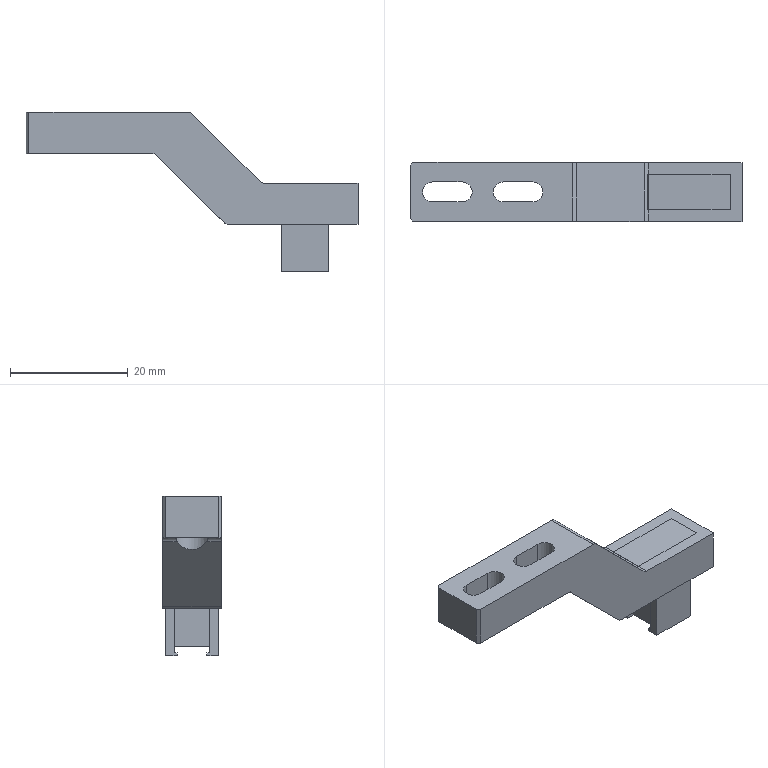NC program | NX | posted with a generic post | part box 56.3 x 10 x 27 mm
Lines 1 to 1605 of 5717:
N10 G17 G21 G94 G90
(FLOOR_WALL , TOOL : D63)
N12 T01 M6
N14 G54
N16 G17 G0 G90 X-65.65 Y0. S6500 M3
N18 G43 Z30. H1
N20 Z3.
N22 G94 G1 Z0. F1250.
N24 X-62.65
N26 X62.65
N28 X65.65
N30 Z3.
N32 G0 Z30.
N34 M5
(ADAPTIVE_MILLING , TOOL : D10)
N36 T10 M6
N38 G54
N40 G17 G0 G90 X-38.845 Y-0.047 S9500 M3
N42 G43 Z30. H10
N44 Z-12.5
N46 G94 G1 Z-13.5 F1000.
N48 X-37.488 Y-0.577 F3000.
N50 G3 X-36.198 Y-0.047 R1.015
N52 X-35.554 Y3.112 R9.424
N54 G2 X-35.341 Y6.202 R38.076
N56 X-31.901 Y10.398 R6.457
N58 X-26.038 Y11.923 R15.304
N60 X-16.444 Y12.181 R121.362
N62 G1 X-14.144 Y12.185
N64 X-9.844 Y12.188
N66 X28.456
N68 X28.556 Y12.187
N70 X28.656 Y12.183
N72 X28.756 Y12.177
N74 G2 X33.079 Y9.425 R5.94
N76 X34.949 Y3.886 R12.695
N78 X35.284 Y-5.899 R69.975
N80 X32.144 Y-10.195 R6.202
N82 X26.729 Y-11.837 R13.656
N84 X17.34 Y-12.177 R88.676
N86 G1 X15.441 Y-12.183
N88 X12.541 Y-12.186
N90 X5.641 Y-12.188
N92 X-28.459
N94 X-28.559 Y-12.187
N96 X-28.659 Y-12.183
N98 G2 X-33.08 Y-9.419 R5.907
N100 X-34.983 Y-3.582 R12.87
N102 X-34.874 Y1.211 R30.869
N104 X-34.492 Y4.48 R15.071
N106 X-30.58 Y9.187 R8.143
N108 X-28.589 Y10.13 R6.111
N110 X-21.397 Y11.234 R26.674
N112 X-8.499 Y11.378 R357.172
N114 G1 X-0.799 Y11.379
N116 X25.701 Y11.38
N118 X25.801 Y11.379
N120 X26.001 Y11.373
N122 X26.101 Y11.369
N124 X26.201 Y11.363
N126 G2 X30.557 Y9.529 R7.732
N128 X33.131 Y6.31 R5.317
N130 X34.353 Y-0.862 R25.486
N132 X34.245 Y-4.246 R11.753
N134 X32.754 Y-7.227 R7.835
N136 X29.553 Y-9.946 R5.116
N138 X22.488 Y-11.192 R25.056
N140 X10.591 Y-11.376 R250.36
N142 G1 X6.191 Y-11.379
N144 X-19.909 Y-11.38
N146 X-25.609
N148 X-25.809 Y-11.378
N150 X-26.009 Y-11.372
N152 X-26.109 Y-11.368
N154 G2 X-31.767 Y-8.166 R7.637
N156 X-33.366 Y-5.037 R6.718
N158 X-33.78 Y2.107 R19.129
N160 X-33.3 Y3.875 R55.35
N162 X-32.568 Y7.13 R6.104
N164 X-30.55 Y9.21 R7.883
N166 G1 X-30.28 Y9.418
N168 X-30.161 Y9.486
N170 G2 X-27.616 Y10.15 R6.048
N172 G3 X-20.523 Y10.444 R251.727
N174 G2 X2.876 Y10.571 R966.744
N176 G1 X23.376
N178 X23.476 Y10.57
N180 X23.676 Y10.566
N182 X23.876 Y10.56
N184 X24.076 Y10.551
N186 G2 X26.44 Y10.15 R13.248
N188 X29.547 Y9.948 R13.204
N190 G1 X30.563 Y9.527
N192 G3 X30.997 Y11.643 R-1.1
N194 G1 X-26.802 Y12.35
N196 G3 X-27.914 Y11.262 R1.1
N198 X-26.816 Y10.15 R1.1
N200 G1 X26.484
N202 G2 X29.547 Y9.948 R13.123
N204 X32.636 Y7.511 R5.459
N206 X33.3 Y4.966 R6.048
N208 G3 X33.512 Y-0.729 R196.858
N210 G2 X33.3 Y-2.654 R13.666
N212 G1 Y-4.966
N214 X33.296 Y-5.034
N216 G2 X32.754 Y-7.228 R5.556
N218 G3 X34.869 Y-7.708 R-1.1
N220 G1 X35.498 Y4.007
N222 G3 X33.3 Y4.066 R-1.1
N224 G1 Y-2.734
N226 X33.296 Y-5.034
N228 G2 X31.834 Y-8.587 R5.543
N230 G1 X31.737 Y-8.683
N232 X30.78 Y-9.418
N234 X30.661 Y-9.486
N236 G2 X28.116 Y-10.15 R6.048
N238 G3 X21.222 Y-10.431 R190.903
N240 G2 X0.124 Y-10.571 R780.86
N242 G1 X-23.376
N244 X-23.576 Y-10.568
N246 X-23.776 Y-10.564
N248 X-23.976 Y-10.556
N250 X-24.076 Y-10.551
N252 G2 X-26.423 Y-10.15 R13.033
N254 X-29.047 Y-9.948 R10.758
N256 X-31.74 Y-8.193 R6.189
N258 G3 X-33.345 Y-8.46 R1.003
N260 X-33.354 Y-9.364 Z-13.454 R1.154
N262 G1 X-33.058 Y-10.391 Z-13.4
N264 X-32.6 Y-11.976
N266 G3 X-31.74 Y-12.693 R1.01
N268 G1 X-25.941 Y-13.27
N270 G3 X-18.669 Y-13.567 R86.44
N272 G1 X20.152 Y-13.459
N274 X22.093 Y-13.405
N276 X24.034 Y-13.332
N278 X24.339 Y-13.272
N280 X26.014 Y-12.656
N282 X27.668 Y-12.042 Z-13.488
N284 X27.864 Y-11.912 Z-13.5
N286 G3 X27.216 Y-10.15 R1.001
N288 G1 X-26.484
N290 G2 X-29.047 Y-9.948 R10.617
N292 X-31.316 Y-8.617 R6.123
N294 X-32.636 Y-7.011 R9.877
N296 X-33.3 Y-4.466 R6.048
N298 G1 Y3.934
N300 G3 X-34.26 Y4.943 R1.015
N302 G1 X-35.75 Y5.016
N304 Z-10.5
N306 G0 Z30.
N308 X11.327 Y12.65
N310 Z-10.849
N312 G1 Z-11.849 F1000.
N314 X11.587 Y10.949 F3000.
N316 G3 X12.449 Y10.102 R1.017
N318 X19.073 Y9.371 R27.652
N320 G2 X26.071 Y9.28 R636.842
N322 X30.346 Y6.274 R6.122
N324 X32.082 Y0.583 R13.598
N326 X32.244 Y-3.007 R17.287
N328 X29.162 Y-7.235 R6.252
N330 X23.367 Y-8.976 R13.982
N332 X14.778 Y-9.319 R99.274
N334 G3 X13.717 Y-9.787 R6.397
N336 G2 X12.119 Y-10.114 R6.107
N338 G3 X12.17 Y-12.109 R1.
N340 G1 X14.166 Y-12.243 Z-11.749
N342 X16.016 Y-12.364
N344 X18.871 Y-12.367
N346 X21.726 Y-12.352
N348 G3 X26.547 Y-11.606 R21.592
N350 X30.515 Y-10.072 R17.224
N352 X33.002 Y-8.113 R10.372
N354 X34.179 Y-6.676 R9.43
N356 X35.307 Y-3.169 R7.965
N358 X35.209 Y1.171 R16.007
N360 G1 X34.962 Y2.662
N362 X34.695 Y4.15
N364 G3 X33.138 Y7.605 R9.851
N366 X30.412 Y10.719 R18.404
N368 X28.184 Y11.912 R6.004
N370 X26.235 Y12.284 R9.527
N372 G1 X16.786 Y13.039
N374 X16.538 Y13.024
N376 X16.298 Y12.955
N378 X14.578 Y12.187
N380 X13.972 Y11.921 Z-11.782
N382 X13.375 Y11.634 Z-11.815
N384 G3 X12.978 Y11.104 Z-11.849 R1.039
N386 X13.604 Y9.857 R1.005
N388 X17.868 Y8.785 R10.881
N390 X23.461 Y8.53 R147.8
N392 G2 X29.401 Y4.439 R7.802
N394 X30.845 Y-0.093 R10.208
N396 X27.704 Y-5.822 R6.984
N398 X21.646 Y-8.007 R13.931
N400 X16.168 Y-8.474 R87.876
N402 G3 X15.531 Y-8.679 R1.836
N404 G2 X14.437 Y-9.432 R5.133
N406 G3 X14.091 Y-10.924 R1.004
N408 X14.885 Y-11.328 Z-11.803 R1.049
N410 G1 X15.958 Y-11.44 Z-11.749
N412 X18.334 Y-11.682
N414 X19.061 Y-11.679
N416 X19.786 Y-11.621
N418 X21.866 Y-11.182
N420 X23.937 Y-10.703
N422 G3 X27.942 Y-9.251 R22.41
N424 G1 X29.435 Y-8.524
N426 G3 X31.337 Y-6.849 R6.438
N428 X32.451 Y-5.198 R13.004
N430 G1 X33.011 Y-4.206
N432 X33.555 Y-3.206
N434 G3 X34.06 Y-0.068 R5.752
N436 X31.366 Y6.799 R14.804
N438 X28.808 Y9.937 R28.114
N440 X27.187 Y10.815 R4.154
N442 G1 X25.826 Y11.157
N444 X24.453 Y11.445
N446 G3 X21.976 Y11.691 R18.706
N448 G1 X20.003 Y11.751
N450 X18.03 Y11.796
N452 X15.86 Y11.573
N454 X15.158 Y11.503 Z-11.784
N456 X14.458 Y11.417 Z-11.82
N458 G3 X13.961 Y11.117 Z-11.849 R1.05
N460 X14.264 Y9.551 R1.003
N462 X15.83 Y8.745 R24.545
N464 X20.746 Y7.928 R18.554
N466 G2 X28.271 Y3.239 R8.723
N468 X27.004 Y-3.629 R6.33
N470 X21.41 Y-6.75 R11.06
N472 X17.087 Y-7.558 R101.827
N474 G3 X15.863 Y-8.391 R1.599
N476 G1 X15.766 Y-8.492
N478 X15.531 Y-8.679
N480 G3 X15.268 Y-9.929 R1.007
N482 X16.077 Y-10.464 Z-11.799 R1.036
N484 G1 X17.052 Y-10.635 Z-11.749
N486 X18.939 Y-10.965
N488 X19.186 Y-10.974
N490 X19.428 Y-10.929
N492 X22.98 Y-9.733
N494 G3 X29.138 Y-5.877 R18.738
N496 X30.944 Y-3.226 R8.435
N498 X31.742 Y-0.891 R11.188
N500 X30.84 Y5.393 R9.525
N502 X29.115 Y7.528 R7.807
N504 G1 X27.376 Y9.014
N506 G3 X24.655 Y10.377 R8.502
N508 G1 X23.934 Y10.572
N510 X23.203 Y10.726
N512 X18.75 Y11.494
N514 X18.585 Y11.504
N516 X18.42 Y11.496
N518 X16.458 Y11.177
N520 X15.812 Y11.077 Z-11.782
N522 X15.171 Y10.952 Z-11.814
N524 G3 X14.643 Y10.525 Z-11.849 R1.038
N526 X14.853 Y9.244 R1.006
N528 X18.143 Y7.67 R6.367
N530 G2 X22.035 Y6.768 R25.917
N532 X25.438 Y4.275 R6.461
N534 X25.152 Y-1.96 R5.738
N536 X20.422 Y-5.494 R9.79
N538 G3 X17.068 Y-6.795 R37.31
N540 X16.518 Y-7.494 R1.478
N542 G1 X16.105 Y-8.06
N544 G3 X16.191 Y-9.341 R1.007
N546 X17.109 Y-9.635 Z-11.799 R1.037
N548 G1 X18.101 Y-9.538 Z-11.749
N550 X19.149 Y-9.439
N552 X20.195 Y-9.325
N554 X20.452 Y-9.224
N556 X22.727 Y-7.932
N558 G3 X25.16 Y-6.205 R22.092
N560 G1 X26.918 Y-4.744
N562 G3 X29.076 Y-0.832 R7.403
N564 X29.376 Y1.612 R10.17
N566 X27.498 Y6.703 R8.238
N568 X25.76 Y8.466 R9.933
N570 X23.236 Y9.781 R8.476
N572 G1 X19.284 Y11.042
N574 X19.045 Y11.084
N576 X18.802 Y11.073
N578 X16.983 Y10.744
N580 X16.334 Y10.631 Z-11.782
N582 X15.69 Y10.495 Z-11.815
N584 G3 X15.175 Y10.067 Z-11.849 R1.039
N586 X15.387 Y8.792 R1.006
N588 X18.269 Y7.139 R6.252
N590 G2 X21.148 Y6.015 R12.282
N592 X23.041 Y0.63 R4.874
N594 X19.898 Y-3.761 R8.375
N596 G3 X17.208 Y-5.834 R31.902
N598 X16.624 Y-7.269 R7.59
N600 X17.043 Y-8.479 R1.007
N602 X18.079 Y-8.496 Z-11.795 R1.107
N604 G1 X18.941 Y-8.176 Z-11.749
N606 X19.921 Y-7.817
N608 X20.895 Y-7.44
N610 X21.124 Y-7.269
N612 X22.967 Y-5.404
N614 G3 X25.383 Y-2.157 R20.777
N616 X26.362 Y2.648 R7.818
N618 X24.501 Y7.531 R10.136
N620 X21.777 Y9.718 R7.181
N622 G1 X20.679 Y10.226
N624 X19.573 Y10.715
N626 G3 X19.016 Y10.718 R1.055
N628 G1 X17.512 Y10.291
N630 X16.853 Y10.108 Z-11.783
N632 X16.199 Y9.906 Z-11.818
N634 G3 X15.745 Y9.483 Z-11.849 R1.044
N636 X15.807 Y8.416 R1.011
N638 X17.817 Y6.823 R4.612
N640 G2 X20.286 Y1.737 R5.054
N642 X18.354 Y-2.813 R9.648
N644 G3 X17.164 Y-4.657 R12.576
N646 G1 X17.139 Y-4.754
N648 X17.121 Y-4.852
N650 X17.118 Y-4.881
N652 Y-4.956
N654 X17.116 Y-5.001
N656 X17.009 Y-6.195
N658 X16.987 Y-6.292
N660 G3 X17.714 Y-7.485 R1.005
N662 X18.706 Y-7.209 Z-11.795 R1.11
N664 G1 X19.45 Y-6.657 Z-11.749
N666 X21.034 Y-5.484
N668 X21.202 Y-5.321
N670 X21.334 Y-5.128
N672 X22.398 Y-2.97
N674 G3 X23.241 Y0.087 R11.085
N676 G1 X23.431 Y1.735
N678 G3 X22.817 Y5.394 R8.433
N680 X21.338 Y8.047 R9.831
N682 G1 X20.82 Y8.712
N684 X20.287 Y9.365
N686 G3 X19.614 Y9.637 R1.03
N688 G1 X18.01 Y9.658
N690 X17.353 Y9.672 Z-11.782
N692 X16.696 Y9.661 Z-11.815
N694 G3 X16.106 Y9.339 Z-11.849 R1.039
N696 X16.041 Y8.091 R1.007
N698 G2 X17.432 Y6.218 R47.2
N700 X18.041 Y0.215 R7.732
N702 X17.129 Y-2.535 R167.132
N704 G1 X17.122 Y-2.592
N706 X17.118 Y-4.892
N708 G3 X19.316 Y-4.827 R-1.1
N710 G1 X18.533 Y8.085
N712 G3 X16.47 Y7.492 R-1.1
N714 G2 X17.233 Y4.116 R7.538
N716 X17.13 Y1.925 R19.575
N718 G1 X17.122 Y-2.675
N720 G3 X19.322 Y-2.659 R-1.1
N722 G1 X19.171 Y6.359
N724 G3 X16.98 Y6.198 R-1.1
N726 G1 X17.131 Y5.041
N728 X17.136 Y4.974
N730 X17.13 Y1.874
N732 G3 X18.063 Y0.866 R1.015
N734 G1 X19.626 Y0.746
N736 Z-8.849
N738 G0 Z30.
N740 X12.358 Y12.55
N742 Z-10.571
N744 G1 Z-11.571 F1000.
N746 X12.151 Y11.813 F3000.
N748 X11.967 Y11.071
N750 G3 X12.715 Y9.984 R1.016
N752 G2 X16.457 Y6.271 R5.331
N754 G1 X16.627 Y5.036
N756 X16.632 Y4.964
N758 Y-4.964
N760 X16.627 Y-5.036
N762 G2 X15.135 Y-8.6 R5.576
N764 X12.841 Y-9.95 R5.798
N766 G3 X12.231 Y-11.082 R1.017
N768 G1 X12.517 Y-12.522
N770 Z-8.571
N772 G0 Z30.
N774 X9.877 Y12.65
N776 Z-9.607
N778 G1 Z-10.607 F1000.
N780 X10.113 Y10.946 F3000.
N782 G3 X10.988 Y10.082 R1.017
N784 G2 X13.101 Y9.429 R5.206
N786 X15.487 Y6.271 R5.495
N788 X15.735 Y2.165 R24.339
N790 X15.716 Y-3.032 R61.356
N792 G3 X15.658 Y-5.036 R13.244
N794 G2 X14.166 Y-8.599 R5.576
N796 X11.725 Y-9.99 R5.74
N798 G1 X10.932 Y-10.09
N800 G3 X10.559 Y-11.949 R1.001
N802 G1 X10.856 Y-12.06 Z-10.591
N804 X11.168 Y-12.118 Z-10.575
N806 X12.511 Y-12.359 Z-10.507
N808 X13.306 Y-12.508
N810 X14.104 Y-12.632
N812 G3 X14.829 Y-12.34 R1.026
N814 G1 X15.86 Y-11.312
N816 X16.878 Y-10.272
N818 G3 X18.16 Y-8.078 R6.848
N820 X18.821 Y-4.92 R11.638
N822 G1 X18.853 Y-4.298
N824 X18.868 Y-3.675
N826 X18.837 Y1.899
N828 X18.782 Y2.126
N830 X18.168 Y3.78
N832 X17.551 Y5.423 Z-10.595
N834 X17.413 Y5.624 Z-10.607
N836 G3 X15.663 Y4.964 R1.001
N838 G1 Y-3.436
N840 G3 X16.539 Y-4.437 R1.015
N842 G1 X18.162 Y-4.654
N844 Z-7.607
N846 G0 Z30.
N848 X8.908 Y12.65
N850 Z-8.643
N852 G1 Z-9.643 F1000.
N854 X9.144 Y10.946 F3000.
N856 G3 X10.018 Y10.082 R1.017
N858 G2 X12.131 Y9.429 R5.206
N860 X14.518 Y6.271 R5.495
N862 X14.765 Y2.165 R24.339
N864 X14.757 Y-2.933 R81.882
N866 G3 X14.688 Y-5.036 R12.32
N868 G2 X13.196 Y-8.599 R5.576
N870 X10.756 Y-9.99 R5.74
N872 G1 X9.962 Y-10.09
N874 G3 X9.589 Y-11.949 R1.001
N876 G1 X9.886 Y-12.06 Z-9.627
N878 X10.198 Y-12.118 Z-9.611
N880 X11.541 Y-12.359 Z-9.543
N882 X12.336 Y-12.508
N884 X13.135 Y-12.632
N886 G3 X13.859 Y-12.34 R1.026
N888 G1 X14.891 Y-11.312
N890 X15.909 Y-10.272
N892 G3 X17.19 Y-8.078 R6.848
N894 X17.851 Y-4.92 R11.638
N896 G1 X17.883 Y-4.298
N898 X17.898 Y-3.675
N900 X17.867 Y1.899
N902 X17.812 Y2.126
N904 X17.199 Y3.78
N906 X16.581 Y5.423 Z-9.631
N908 X16.444 Y5.624 Z-9.643
N910 G3 X14.693 Y4.964 R1.001
N912 G1 Y-3.336
N914 G3 X15.583 Y-4.339 R1.015
N916 G1 X17.193 Y-4.53
N918 Z-6.643
N920 G0 Z30.
N922 X7.938 Y12.65
N924 Z-7.679
N926 G1 Z-8.679 F1000.
N928 X8.174 Y10.946 F3000.
N930 G3 X9.049 Y10.082 R1.017
N932 G2 X11.161 Y9.429 R5.206
N934 X13.548 Y6.271 R5.495
N936 X13.795 Y2.165 R24.338
N938 X13.787 Y-2.933 R81.882
N940 G3 X13.718 Y-5.036 R12.316
N942 G2 X12.226 Y-8.6 R5.576
N944 X9.786 Y-9.99 R5.74
N946 G1 X8.992 Y-10.09
N948 G3 X8.619 Y-11.949 R1.001
N950 G1 X8.916 Y-12.06 Z-8.663
N952 X9.228 Y-12.118 Z-8.647
N954 X10.571 Y-12.359 Z-8.579
N956 X11.366 Y-12.508
N958 X12.165 Y-12.632
N960 G3 X12.889 Y-12.34 R1.026
N962 G1 X13.921 Y-11.312
N964 X14.939 Y-10.272
N966 G3 X16.22 Y-8.078 R6.848
N968 X16.882 Y-4.92 R11.638
N970 G1 X16.913 Y-4.298
N972 X16.928 Y-3.675
N974 X16.898 Y1.899
N976 X16.843 Y2.126
N978 X16.229 Y3.78
N980 X15.611 Y5.423 Z-8.666
N982 X15.474 Y5.624 Z-8.679
N984 G3 X13.723 Y4.964 R1.001
N986 G1 Y-3.336
N988 G3 X14.614 Y-4.339 R1.015
N990 G1 X16.223 Y-4.53
N992 Z-5.679
N994 G0 Z30.
N996 X6.968 Y12.65
N998 Z-6.714
N1000 G1 Z-7.714 F1000.
N1002 X7.204 Y10.946 F3000.
N1004 G3 X8.079 Y10.082 R1.017
N1006 G2 X10.192 Y9.429 R5.206
N1008 X12.578 Y6.271 R5.495
N1010 X12.826 Y2.165 R24.339
N1012 X12.807 Y-3.032 R61.356
N1014 G3 X12.748 Y-5.036 R13.234
N1016 G2 X11.256 Y-8.6 R5.576
N1018 X8.816 Y-9.99 R5.74
N1020 G1 X8.022 Y-10.09
N1022 G3 X7.65 Y-11.949 R1.001
N1024 G1 X7.947 Y-12.06 Z-7.698
N1026 X8.258 Y-12.118 Z-7.683
N1028 X9.601 Y-12.359 Z-7.614
N1030 X10.396 Y-12.508
N1032 X11.195 Y-12.632
N1034 G3 X11.919 Y-12.34 R1.026
N1036 G1 X12.951 Y-11.312
N1038 X13.969 Y-10.272
N1040 G3 X15.251 Y-8.078 R6.848
N1042 X15.912 Y-4.92 R11.638
N1044 G1 X15.944 Y-4.298
N1046 X15.959 Y-3.675
N1048 X15.928 Y1.899
N1050 X15.873 Y2.126
N1052 X15.259 Y3.78
N1054 X14.642 Y5.423 Z-7.702
N1056 X14.504 Y5.624 Z-7.714
N1058 G3 X12.753 Y4.964 R1.001
N1060 G1 Y-3.436
N1062 G3 X13.63 Y-4.437 R1.015
N1064 G1 X15.253 Y-4.654
N1066 Z-4.714
N1068 G0 Z30.
N1070 X5.998 Y12.65
N1072 Z-5.75
N1074 G1 Z-6.75 F1000.
N1076 X6.234 Y10.946 F3000.
N1078 G3 X7.109 Y10.082 R1.017
N1080 G2 X9.222 Y9.429 R5.206
N1082 X11.608 Y6.271 R5.495
N1084 X11.856 Y2.165 R24.338
N1086 X11.837 Y-3.032 R61.356
N1088 G3 X11.779 Y-5.036 R13.238
N1090 G2 X10.287 Y-8.6 R5.576
N1092 X7.846 Y-9.99 R5.74
N1094 G1 X7.053 Y-10.09
N1096 G3 X6.68 Y-11.949 R1.001
N1098 G1 X6.977 Y-12.06 Z-6.734
N1100 X7.289 Y-12.118 Z-6.718
N1102 X8.632 Y-12.359 Z-6.65
N1104 X9.426 Y-12.508
N1106 X10.225 Y-12.632
N1108 G3 X10.95 Y-12.34 R1.026
N1110 G1 X11.981 Y-11.312
N1112 X12.999 Y-10.272
N1114 G3 X14.281 Y-8.078 R6.848
N1116 X14.942 Y-4.92 R11.638
N1118 G1 X14.974 Y-4.298
N1120 X14.989 Y-3.675
N1122 X14.958 Y1.899
N1124 X14.903 Y2.126
N1126 X14.289 Y3.78
N1128 X13.672 Y5.423 Z-6.738
N1130 X13.535 Y5.624 Z-6.75
N1132 G3 X11.784 Y4.964 R1.001
N1134 G1 Y-3.436
N1136 G3 X12.66 Y-4.437 R1.015
N1138 G1 X14.283 Y-4.654
N1140 Z-3.75
N1142 G0 Z30.
N1144 X5.028 Y12.65
N1146 Z-4.786
N1148 G1 Z-5.786 F1000.
N1150 X5.264 Y10.946 F3000.
N1152 G3 X6.139 Y10.082 R1.017
N1154 G2 X8.252 Y9.429 R5.206
N1156 X10.639 Y6.271 R5.495
N1158 X10.886 Y2.165 R24.339
N1160 X10.867 Y-3.032 R61.311
N1162 G3 X10.809 Y-5.036 R13.25
N1164 G2 X9.317 Y-8.6 R5.576
N1166 X6.877 Y-9.99 R5.74
N1168 G1 X6.083 Y-10.09
N1170 G3 X5.71 Y-11.949 R1.001
N1172 G1 X6.007 Y-12.06 Z-5.77
N1174 X6.319 Y-12.118 Z-5.754
N1176 X7.662 Y-12.359 Z-5.686
N1178 X8.457 Y-12.508
N1180 X9.256 Y-12.632
N1182 G3 X9.98 Y-12.34 R1.026
N1184 G1 X11.012 Y-11.312
N1186 X12.029 Y-10.272
N1188 G3 X13.311 Y-8.078 R6.848
N1190 X13.972 Y-4.92 R11.638
N1192 G1 X14.004 Y-4.298
N1194 X14.019 Y-3.675
N1196 X13.988 Y1.899
N1198 X13.933 Y2.126
N1200 X13.32 Y3.78
N1202 X12.702 Y5.423 Z-5.774
N1204 X12.565 Y5.624 Z-5.786
N1206 G3 X10.814 Y4.964 R1.001
N1208 G1 Y-3.436
N1210 G3 X11.69 Y-4.437 R1.015
N1212 G1 X13.314 Y-4.654
N1214 Z-2.786
N1216 G0 Z30.
N1218 X4.059 Y12.65
N1220 Z-3.821
N1222 G1 Z-4.821 F1000.
N1224 X4.295 Y10.946 F3000.
N1226 G3 X5.17 Y10.082 R1.017
N1228 G2 X7.282 Y9.429 R5.206
N1230 X9.669 Y6.271 R5.495
N1232 X9.916 Y2.165 R24.338
N1234 X9.908 Y-2.933 R81.882
N1236 G3 X9.839 Y-5.036 R12.316
N1238 G2 X8.347 Y-8.6 R5.576
N1240 X5.907 Y-9.99 R5.74
N1242 G1 X5.113 Y-10.09
N1244 G3 X4.741 Y-11.949 R1.001
N1246 G1 X5.037 Y-12.06 Z-4.806
N1248 X5.349 Y-12.118 Z-4.79
N1250 X6.692 Y-12.359 Z-4.721
N1252 X7.487 Y-12.508
N1254 X8.286 Y-12.632
N1256 G3 X9.01 Y-12.34 R1.026
N1258 G1 X10.042 Y-11.312
N1260 X11.06 Y-10.272
N1262 G3 X12.341 Y-8.078 R6.848
N1264 X13.003 Y-4.92 R11.638
N1266 G1 X13.035 Y-4.298
N1268 X13.049 Y-3.675
N1270 X13.019 Y1.899
N1272 X12.964 Y2.126
N1274 X12.35 Y3.78
N1276 X11.732 Y5.423 Z-4.809
N1278 X11.595 Y5.624 Z-4.821
N1280 G3 X9.844 Y4.964 R1.001
N1282 G1 Y-3.336
N1284 G3 X10.735 Y-4.339 R1.015
N1286 G1 X12.344 Y-4.53
N1288 Z-1.821
N1290 G0 Z30.
N1292 X3.089 Y12.65
N1294 Z-2.857
N1296 G1 Z-3.857 F1000.
N1298 X3.325 Y10.946 F3000.
N1300 G3 X4.2 Y10.082 R1.017
N1302 G2 X6.313 Y9.429 R5.206
N1304 X8.699 Y6.271 R5.495
N1306 X8.947 Y2.165 R24.338
N1308 X8.928 Y-3.032 R61.356
N1310 G3 X8.869 Y-5.036 R13.238
N1312 G2 X7.378 Y-8.6 R5.576
N1314 X4.937 Y-9.99 R5.74
N1316 G1 X4.143 Y-10.09
N1318 G3 X3.771 Y-11.949 R1.001
N1320 G1 X4.068 Y-12.06 Z-3.841
N1322 X4.379 Y-12.118 Z-3.825
N1324 X5.722 Y-12.359 Z-3.757
N1326 X6.517 Y-12.508
N1328 X7.316 Y-12.632
N1330 G3 X8.041 Y-12.34 R1.026
N1332 G1 X9.072 Y-11.312
N1334 X10.09 Y-10.272
N1336 G3 X11.372 Y-8.078 R6.848
N1338 X12.033 Y-4.92 R11.638
N1340 G1 X12.065 Y-4.298
N1342 X12.08 Y-3.675
N1344 X12.049 Y1.899
N1346 X11.994 Y2.126
N1348 X11.38 Y3.78
N1350 X10.763 Y5.423 Z-3.845
N1352 X10.625 Y5.624 Z-3.857
N1354 G3 X8.874 Y4.964 R1.001
N1356 G1 Y-3.436
N1358 G3 X9.751 Y-4.437 R1.015
N1360 G1 X11.374 Y-4.654
N1362 Z-0.857
N1364 G0 Z30.
N1366 X2.119 Y12.65
N1368 Z-1.893
N1370 G1 Z-2.893 F1000.
N1372 X2.355 Y10.946 F3000.
N1374 G3 X3.23 Y10.082 R1.017
N1376 G2 X5.343 Y9.429 R5.206
N1378 X7.729 Y6.271 R5.495
N1380 X7.977 Y2.165 R24.338
N1382 X7.969 Y-2.933 R81.882
N1384 G3 X7.9 Y-5.036 R12.317
N1386 G2 X6.408 Y-8.599 R5.576
N1388 X3.967 Y-9.99 R5.74
N1390 G1 X3.174 Y-10.09
N1392 G3 X2.801 Y-11.949 R1.001
N1394 G1 X3.098 Y-12.06 Z-2.877
N1396 X3.41 Y-12.118 Z-2.861
N1398 X4.753 Y-12.359 Z-2.793
N1400 X5.548 Y-12.508
N1402 X6.346 Y-12.632
N1404 G3 X7.071 Y-12.34 R1.026
N1406 G1 X8.102 Y-11.312
N1408 X9.12 Y-10.272
N1410 G3 X10.402 Y-8.078 R6.848
N1412 X11.063 Y-4.92 R11.638
N1414 G1 X11.095 Y-4.298
N1416 X11.11 Y-3.675
N1418 X11.079 Y1.899
N1420 X11.024 Y2.126
N1422 X10.41 Y3.78
N1424 X9.793 Y5.423 Z-2.881
N1426 X9.656 Y5.624 Z-2.893
N1428 G3 X7.905 Y4.964 R1.001
N1430 G1 Y-3.336
N1432 G3 X8.795 Y-4.339 R1.015
N1434 G1 X10.404 Y-4.53
N1436 Z0.107
N1438 G0 Z30.
N1440 X1.149 Y12.65
N1442 Z-0.929
N1444 G1 Z-1.929 F1000.
N1446 X1.385 Y10.946 F3000.
N1448 G3 X2.26 Y10.082 R1.017
N1450 G2 X4.373 Y9.429 R5.206
N1452 X6.76 Y6.271 R5.495
N1454 X7.007 Y2.165 R24.339
N1456 X6.988 Y-3.032 R61.311
N1458 G3 X6.93 Y-5.036 R13.25
N1460 G2 X5.438 Y-8.6 R5.576
N1462 X2.998 Y-9.99 R5.74
N1464 G1 X2.204 Y-10.09
N1466 G3 X1.831 Y-11.949 R1.001
N1468 G1 X2.128 Y-12.06 Z-1.913
N1470 X2.44 Y-12.118 Z-1.897
N1472 X3.783 Y-12.359 Z-1.829
N1474 X4.578 Y-12.508
N1476 X5.377 Y-12.632
N1478 G3 X6.101 Y-12.34 R1.026
N1480 G1 X7.133 Y-11.312
N1482 X8.151 Y-10.272
N1484 G3 X9.432 Y-8.078 R6.848
N1486 X10.093 Y-4.92 R11.638
N1488 G1 X10.125 Y-4.298
N1490 X10.14 Y-3.675
N1492 X10.11 Y1.899
N1494 X10.054 Y2.126
N1496 X9.441 Y3.78
N1498 X8.823 Y5.423 Z-1.916
N1500 X8.686 Y5.624 Z-1.929
N1502 G3 X6.935 Y4.964 R1.001
N1504 G1 Y-3.436
N1506 G3 X7.811 Y-4.437 R1.015
N1508 G1 X9.435 Y-4.654
N1510 Z1.071
N1512 G0 Z30.
N1514 X-38.846 Y-0.049
N1516 Z-26.
N1518 G1 Z-27. F1000.
N1520 X-37.49 Y-0.579 F3000.
N1522 G3 X-36.2 Y-0.049 R1.015
N1524 X-35.556 Y3.111 R9.424
N1526 G2 X-35.343 Y6.201 R38.076
N1528 X-31.904 Y10.397 R6.451
N1530 X-25.942 Y11.933 R15.338
N1532 X-16.248 Y12.183 R123.656
N1534 G1 X-13.748 Y12.187
N1536 X-8.948 Y12.19
N1538 X28.452
N1540 X28.552 Y12.189
N1542 X28.652 Y12.185
N1544 X28.752 Y12.18
N1546 G2 X33.078 Y9.431 R5.943
N1548 X34.937 Y3.992 R12.564
N1550 X35.286 Y-5.892 R69.411
N1552 X32.153 Y-10.192 R6.2
N1554 X26.442 Y-11.872 R14.005
N1556 X17.251 Y-12.18 R95.383
N1558 G1 X15.351 Y-12.185
N1560 X12.351 Y-12.188
N1562 X4.751 Y-12.19
N1564 X-28.449
N1566 X-28.549 Y-12.189
N1568 X-28.649 Y-12.185
N1570 G2 X-33.019 Y-9.516 R5.866
N1572 X-34.95 Y-3.896 R12.546
N1574 X-34.883 Y1.096 R27.12
N1576 X-34.499 Y4.466 R16.044
N1578 X-30.567 Y9.197 R8.146
N1580 X-28.59 Y10.131 R6.145
N1582 X-21.698 Y11.223 R25.96
N1584 X-7.2 Y11.38 R368.658
N1586 G1 X5.4 Y11.381
N1588 X25.7
N1590 X25.8
N1592 X26. Y11.375
N1594 X26.1 Y11.37
N1596 X26.2 Y11.364
N1598 G2 X30.557 Y9.53 R7.734
N1600 X33.133 Y6.31 R5.33
N1602 X34.368 Y-1.06 R26.109
N1604 X34.174 Y-4.536 R10.342
N1606 X32.748 Y-7.243 R8.16
N1608 X29.46 Y-9.981 R5.174
N1610 X22.189 Y-11.211 R25.756
N1612 X9.392 Y-11.379 R301.168
N1614 G1 X3.392 Y-11.381
N1616 X-25.608
N1618 X-25.808 Y-11.38
N1620 X-26.008 Y-11.374
N1622 X-26.208 Y-11.364
N1624 G2 X-31.767 Y-8.166 R7.583
N1626 X-33.366 Y-5.038 R6.73
N1628 X-33.785 Y2.107 R19.114
N1630 X-33.3 Y3.886 R65.462
N1632 X-32.568 Y7.13 R6.094
N1634 X-30.55 Y9.21 R7.883
N1636 G1 X-30.28 Y9.418
N1638 X-30.161 Y9.486
N1640 G2 X-26.916 Y10.15 R6.283
N1642 X-8.424 Y10.569 R289.04
N1644 G1 X-4.024 Y10.572
N1646 X12.076 Y10.573
N1648 X23.376 Y10.572
N1650 X23.576 Y10.57
N1652 X23.776 Y10.566
N1654 X23.976 Y10.558
N1656 G2 X26.448 Y10.15 R12.614
N1658 X29.547 Y9.948 R13.159
N1660 G1 X30.563 Y9.527
N1662 G3 X30.997 Y11.643 R-1.1
N1664 G1 X-26.902 Y12.35
N1666 G3 X-28.014 Y11.262 R1.1
N1668 X-26.916 Y10.15 R1.1
N1670 G1 X26.484
N1672 G2 X29.547 Y9.948 R13.123
N1674 X32.636 Y7.511 R5.459
N1676 X33.3 Y4.966 R6.048
N1678 G3 X33.516 Y-0.729 R198.709
N1680 G2 X33.3 Y-2.682 R13.343
N1682 X33.134 Y-6.265 R18.221
N1684 G1 X33.098 Y-6.397
N1686 X32.716 Y-7.32
N1688 G3 X34.83 Y-7.803 R-1.1
N1690 G1 X35.498 Y4.003
N1692 G3 X33.3 Y4.066 R-1.1
N1694 G1 Y-2.734
N1696 X33.296 Y-5.034
N1698 G2 X31.834 Y-8.587 R5.543
N1700 G1 X31.737 Y-8.683
N1702 X30.78 Y-9.418
N1704 X30.661 Y-9.486
N1706 G2 X28.116 Y-10.15 R6.048
N1708 G3 X20.923 Y-10.442 R221.959
N1710 G2 X2.624 Y-10.572 R745.337
N1712 G1 X-23.376
N1714 X-23.576 Y-10.57
N1716 X-23.776 Y-10.566
N1718 X-23.976 Y-10.558
N1720 X-24.076 Y-10.553
N1722 G2 X-26.431 Y-10.15 R13.277
N1724 X-29.047 Y-9.948 R10.72
N1726 X-31.74 Y-8.193 R6.189
N1728 G3 X-33.345 Y-8.46 R1.003
N1730 X-33.354 Y-9.364 Z-26.954 R1.154
N1732 G1 X-33.058 Y-10.391 Z-26.9
N1734 X-32.6 Y-11.976
N1736 G3 X-31.74 Y-12.693 R1.01
N1738 G1 X-25.941 Y-13.27
N1740 G3 X-18.669 Y-13.567 R86.44
N1742 G1 X20.152 Y-13.459
N1744 X22.093 Y-13.405
N1746 X24.034 Y-13.332
N1748 X24.339 Y-13.272
N1750 X26.014 Y-12.656
N1752 X27.668 Y-12.042 Z-26.988
N1754 X27.864 Y-11.912 Z-27.
N1756 G3 X27.216 Y-10.15 R1.001
N1758 G1 X-26.484
N1760 G2 X-29.047 Y-9.948 R10.617
N1762 X-31.316 Y-8.617 R6.123
N1764 X-32.636 Y-7.011 R9.877
N1766 X-33.3 Y-4.466 R6.048
N1768 G1 Y3.934
N1770 G3 X-34.26 Y4.943 R1.015
N1772 G1 X-35.75 Y5.016
N1774 Z-24.
N1776 G0 Z30.
N1778 M5
(ZLEVEL_PROFILE_COPY_COPY_1 , TOOL : D10JING)
N1780 T11 M6
N1782 G54
N1784 G17 G0 G90 X-28.477 Y10.438 S9500 M3
N1786 G43 Z30. H11
N1788 Z-10.5
N1790 G94 G1 Z-13.5 F1200.
N1792 G3 X-27.65 Y10. R1.
N1794 G1 X28.15
N1796 G2 X33.15 Y5. R5.
N1798 G1 Y-5.
N1800 G2 X28.15 Y-10. R5.
N1802 G1 X-27.65
N1804 G2 X-31.186 Y-8.536 R5.
N1806 G1 X-31.686 Y-8.036
N1808 G2 X-33.15 Y-4.5 R5.
N1810 G1 Y4.5
N1812 G2 X-31.686 Y8.036 R5.
N1814 G1 X-31.186 Y8.536
N1816 G2 X-27.65 Y10. R5.
N1818 G3 X-26.784 Y10.5 R1.
N1820 G1 Z-10.5
N1822 G0 Z30.
N1824 X-28.477 Y10.438
N1826 Z-24.
N1828 G1 Z-27.
N1830 G3 X-27.65 Y10. R1.
N1832 G1 X28.15
N1834 G2 X33.15 Y5. R5.
N1836 G1 Y-5.
N1838 G2 X28.15 Y-10. R5.
N1840 G1 X-27.65
N1842 G2 X-31.186 Y-8.536 R5.
N1844 G1 X-31.686 Y-8.036
N1846 G2 X-33.15 Y-4.5 R5.
N1848 G1 Y4.5
N1850 G2 X-31.686 Y8.036 R5.
N1852 G1 X-31.186 Y8.536
N1854 G2 X-27.65 Y10. R5.
N1856 G3 X-26.784 Y10.5 R1.
N1858 G1 Z-24.
N1860 G0 Z30.
N1862 M5
(FLOOR_WALL_1 , TOOL : D6)
N1864 T06 M6
N1866 G54
N1868 G17 G0 G90 X32.273 Y8.995 S9500 M3
N1870 G43 Z30. H6
N1872 Z-10.5
N1874 G94 G1 Z-12. F1250.
N1876 X31.45 Y8.52
N1878 G3 X31.15 Y8. R0.6
N1880 G1 Y-8.
N1882 X28.552
N1884 Y8.
N1886 X25.954
N1888 Y-8.
N1890 X23.357
N1892 Y8.
N1894 X20.759
N1896 Y-8.
N1898 X18.161
N1900 Y8.
N1902 X15.563
N1904 Y-8.
N1906 G3 X15.863 Y-8.52 R0.6
N1908 G1 X17.561 Y-9.5
N1910 Z-10.5
N1912 G0 Z30.
N1914 X17.261 Y9.5
N1916 Z-10.5
N1918 G1 Z-12.
N1920 X15.563 Y8.52
N1922 G3 X15.263 Y8. R0.6
N1924 G1 Y0.
N1926 X15.15
N1928 X15.263
N1930 Y-8.
N1932 G3 X15.563 Y-8.52 R0.6
N1934 G1 X17.261 Y-9.5
N1936 Z-10.5
N1938 G0 Z30.
N1940 M5
(ZLEVEL_PROFILE , TOOL : D4)
N1942 T04 M6
N1944 G54
N1946 G17 G0 G90 X22.642 Y0.9 S9500 M3
N1948 G43 Z30. H4
N1950 Z-10.5
N1952 G94 G1 X14.25 Z-10.94 F800.
N1954 Y-0.9 Z-11.034
N1956 X24.05 Z-11.548
N1958 Y0.9 Z-11.642
N1960 X14.25 Z-12.156
N1962 Y-0.9 Z-12.25
N1964 X24.05 F2000.
N1966 Y0.9
N1968 X14.25
N1970 Y-0.9
N1972 X23.939 Z-12.419
N1974 X24.05 Y-0.871 Z-12.422
N1976 Y0.814 Z-12.451
N1978 X23.995 Y0.9 Z-12.453
N1980 X21.328 Z-12.5
N1982 X14.25
N1984 Y-0.9
N1986 X23.939 Z-12.669
N1988 X24.05 Y-0.871 Z-12.672
N1990 Y0.814 Z-12.701
N1992 X23.995 Y0.9 Z-12.703
N1994 X21.328 Z-12.75
N1996 X14.25
N1998 Y-0.9
N2000 X23.939 Z-12.919
N2002 X24.05 Y-0.871 Z-12.922
N2004 Y0.814 Z-12.951
N2006 X23.995 Y0.9 Z-12.953
N2008 X21.328 Z-13.
N2010 X14.25
N2012 Y-0.9
N2014 X23.939 Z-13.169
N2016 X24.05 Y-0.871 Z-13.172
N2018 Y0.814 Z-13.201
N2020 X23.995 Y0.9 Z-13.203
N2022 X21.328 Z-13.25
N2024 X14.25
N2026 Y-0.9
N2028 X23.939 Z-13.419
N2030 X24.05 Y-0.871 Z-13.422
N2032 Y0.814 Z-13.451
N2034 X23.995 Y0.9 Z-13.453
N2036 X21.328 Z-13.5
N2038 X14.25
N2040 Y-0.9
N2042 X23.939 Z-13.669
N2044 X24.05 Y-0.871 Z-13.672
N2046 Y0.814 Z-13.701
N2048 X23.995 Y0.9 Z-13.703
N2050 X21.328 Z-13.75
N2052 X14.25
N2054 Y-0.9
N2056 X23.939 Z-13.919
N2058 X24.05 Y-0.871 Z-13.922
N2060 Y0.814 Z-13.951
N2062 X23.995 Y0.9 Z-13.953
N2064 X21.328 Z-14.
N2066 X14.25
N2068 Y-0.9
N2070 X23.939 Z-14.169
N2072 X24.05 Y-0.871 Z-14.172
N2074 Y0.814 Z-14.201
N2076 X23.995 Y0.9 Z-14.203
N2078 X21.328 Z-14.25
N2080 X14.25
N2082 Y-0.9
N2084 X23.939 Z-14.419
N2086 X24.05 Y-0.871 Z-14.422
N2088 Y0.814 Z-14.451
N2090 X23.995 Y0.9 Z-14.453
N2092 X21.328 Z-14.5
N2094 X14.25
N2096 Y-0.9
N2098 X23.939 Z-14.669
N2100 X24.05 Y-0.871 Z-14.672
N2102 Y0.814 Z-14.701
N2104 X23.995 Y0.9 Z-14.703
N2106 X21.328 Z-14.75
N2108 X14.25
N2110 Y-0.9
N2112 X23.939 Z-14.919
N2114 X24.05 Y-0.871 Z-14.922
N2116 Y0.814 Z-14.951
N2118 X23.995 Y0.9 Z-14.953
N2120 X21.328 Z-15.
N2122 X14.25
N2124 Y-0.9
N2126 X23.939 Z-15.169
N2128 X24.05 Y-0.871 Z-15.172
N2130 Y0.814 Z-15.201
N2132 X23.995 Y0.9 Z-15.203
N2134 X21.328 Z-15.25
N2136 X14.25
N2138 Y-0.9
N2140 X23.939 Z-15.419
N2142 X24.05 Y-0.871 Z-15.422
N2144 Y0.814 Z-15.451
N2146 X23.995 Y0.9 Z-15.453
N2148 X21.328 Z-15.5
N2150 X14.25
N2152 Y-0.9
N2154 X23.939 Z-15.669
N2156 X24.05 Y-0.871 Z-15.672
N2158 Y0.814 Z-15.701
N2160 X23.995 Y0.9 Z-15.703
N2162 X21.328 Z-15.75
N2164 X14.25
N2166 Y-0.9
N2168 X23.939 Z-15.919
N2170 X24.05 Y-0.871 Z-15.922
N2172 Y0.814 Z-15.951
N2174 X23.995 Y0.9 Z-15.953
N2176 X21.328 Z-16.
N2178 X14.25
N2180 Y-0.9
N2182 X23.939 Z-16.169
N2184 X24.05 Y-0.871 Z-16.172
N2186 Y0.814 Z-16.201
N2188 X23.995 Y0.9 Z-16.203
N2190 X21.328 Z-16.25
N2192 X14.25
N2194 Y-0.9
N2196 X23.939 Z-16.419
N2198 X24.05 Y-0.871 Z-16.422
N2200 Y0.814 Z-16.451
N2202 X23.995 Y0.9 Z-16.453
N2204 X21.328 Z-16.5
N2206 X14.25
N2208 Y-0.9
N2210 X23.939 Z-16.669
N2212 X24.05 Y-0.871 Z-16.672
N2214 Y0.814 Z-16.701
N2216 X23.995 Y0.9 Z-16.703
N2218 X21.328 Z-16.75
N2220 X14.25
N2222 Y-0.9
N2224 X23.939 Z-16.919
N2226 X24.05 Y-0.871 Z-16.922
N2228 Y0.814 Z-16.951
N2230 X23.995 Y0.9 Z-16.953
N2232 X21.328 Z-17.
N2234 X14.25
N2236 Y-0.9
N2238 X23.939 Z-17.169
N2240 X24.05 Y-0.871 Z-17.172
N2242 Y0.814 Z-17.201
N2244 X23.995 Y0.9 Z-17.203
N2246 X21.328 Z-17.25
N2248 X14.25
N2250 Y-0.9
N2252 X23.939 Z-17.419
N2254 X24.05 Y-0.871 Z-17.422
N2256 Y0.814 Z-17.451
N2258 X23.995 Y0.9 Z-17.453
N2260 X21.328 Z-17.5
N2262 X14.25
N2264 Y-0.9
N2266 X23.939 Z-17.669
N2268 X24.05 Y-0.871 Z-17.672
N2270 Y0.814 Z-17.701
N2272 X23.995 Y0.9 Z-17.703
N2274 X21.328 Z-17.75
N2276 X14.25
N2278 Y-0.9
N2280 X23.939 Z-17.919
N2282 X24.05 Y-0.871 Z-17.922
N2284 Y0.814 Z-17.951
N2286 X23.995 Y0.9 Z-17.953
N2288 X21.328 Z-18.
N2290 X14.25
N2292 Y-0.9
N2294 X23.939 Z-18.169
N2296 X24.05 Y-0.871 Z-18.172
N2298 Y0.814 Z-18.201
N2300 X23.995 Y0.9 Z-18.203
N2302 X21.328 Z-18.25
N2304 X14.25
N2306 Y-0.9
N2308 X23.939 Z-18.419
N2310 X24.05 Y-0.871 Z-18.422
N2312 Y0.814 Z-18.451
N2314 X23.995 Y0.9 Z-18.453
N2316 X21.328 Z-18.5
N2318 X14.25
N2320 Y-0.9
N2322 X23.939 Z-18.669
N2324 X24.05 Y-0.871 Z-18.672
N2326 Y0.814 Z-18.701
N2328 X23.995 Y0.9 Z-18.703
N2330 X21.328 Z-18.75
N2332 X14.25
N2334 Y-0.9
N2336 X23.939 Z-18.919
N2338 X24.05 Y-0.871 Z-18.922
N2340 Y0.814 Z-18.951
N2342 X23.995 Y0.9 Z-18.953
N2344 X21.328 Z-19.
N2346 X14.25
N2348 Y-0.9
N2350 X23.939 Z-19.169
N2352 X24.05 Y-0.871 Z-19.172
N2354 Y0.814 Z-19.201
N2356 X23.995 Y0.9 Z-19.203
N2358 X21.328 Z-19.25
N2360 X14.25
N2362 Y-0.9
N2364 X23.939 Z-19.419
N2366 X24.05 Y-0.871 Z-19.422
N2368 Y0.814 Z-19.451
N2370 X23.995 Y0.9 Z-19.453
N2372 X21.328 Z-19.5
N2374 X14.25
N2376 Y-0.9
N2378 X23.939 Z-19.669
N2380 X24.05 Y-0.871 Z-19.672
N2382 Y0.814 Z-19.701
N2384 X23.995 Y0.9 Z-19.703
N2386 X21.328 Z-19.75
N2388 X14.25
N2390 Y-0.9
N2392 X23.939 Z-19.919
N2394 X24.05 Y-0.871 Z-19.922
N2396 Y0.814 Z-19.951
N2398 X23.995 Y0.9 Z-19.953
N2400 X21.328 Z-20.
N2402 X14.25
N2404 Y-0.9
N2406 X23.939 Z-20.169
N2408 X24.05 Y-0.871 Z-20.172
N2410 Y0.814 Z-20.201
N2412 X23.995 Y0.9 Z-20.203
N2414 X21.328 Z-20.25
N2416 X14.25
N2418 Y-0.9
N2420 X23.939 Z-20.419
N2422 X24.05 Y-0.871 Z-20.422
N2424 Y0.814 Z-20.451
N2426 X23.995 Y0.9 Z-20.453
N2428 X21.328 Z-20.5
N2430 X14.25
N2432 Y-0.9
N2434 X23.939 Z-20.669
N2436 X24.05 Y-0.871 Z-20.672
N2438 Y0.814 Z-20.701
N2440 X23.995 Y0.9 Z-20.703
N2442 X21.328 Z-20.75
N2444 X14.25
N2446 Y-0.9
N2448 X23.939 Z-20.919
N2450 X24.05 Y-0.871 Z-20.922
N2452 Y0.814 Z-20.951
N2454 X23.995 Y0.9 Z-20.953
N2456 X21.328 Z-21.
N2458 X14.25
N2460 Y-0.9
N2462 X23.939 Z-21.169
N2464 X24.05 Y-0.871 Z-21.172
N2466 Y0.814 Z-21.201
N2468 X23.995 Y0.9 Z-21.203
N2470 X21.328 Z-21.25
N2472 X14.25
N2474 Y-0.9
N2476 X23.939 Z-21.419
N2478 X24.05 Y-0.871 Z-21.422
N2480 Y0.814 Z-21.451
N2482 X23.995 Y0.9 Z-21.453
N2484 X21.328 Z-21.5
N2486 X14.25
N2488 Y-0.9
N2490 X23.939 Z-21.669
N2492 X24.05 Y-0.871 Z-21.672
N2494 Y0.814 Z-21.701
N2496 X23.995 Y0.9 Z-21.703
N2498 X21.328 Z-21.75
N2500 X14.25
N2502 Y-0.9
N2504 X23.939 Z-21.919
N2506 X24.05 Y-0.871 Z-21.922
N2508 Y0.814 Z-21.951
N2510 X23.995 Y0.9 Z-21.953
N2512 X21.328 Z-22.
N2514 X14.25
N2516 Y-0.9
N2518 X23.939 Z-22.169
N2520 X24.05 Y-0.871 Z-22.172
N2522 Y0.814 Z-22.201
N2524 X23.995 Y0.9 Z-22.203
N2526 X21.328 Z-22.25
N2528 X14.25
N2530 Y-0.9
N2532 X23.939 Z-22.419
N2534 X24.05 Y-0.871 Z-22.422
N2536 Y0.814 Z-22.451
N2538 X23.995 Y0.9 Z-22.453
N2540 X21.328 Z-22.5
N2542 X14.25
N2544 Y-0.9
N2546 X23.939 Z-22.669
N2548 X24.05 Y-0.871 Z-22.672
N2550 Y0.814 Z-22.701
N2552 X23.995 Y0.9 Z-22.703
N2554 X21.328 Z-22.75
N2556 X14.25
N2558 Y-0.9
N2560 X23.939 Z-22.919
N2562 X24.05 Y-0.871 Z-22.922
N2564 Y0.814 Z-22.951
N2566 X23.995 Y0.9 Z-22.953
N2568 X21.328 Z-23.
N2570 X14.25
N2572 Y-0.9
N2574 X23.939 Z-23.169
N2576 X24.05 Y-0.871 Z-23.172
N2578 Y0.814 Z-23.201
N2580 X23.995 Y0.9 Z-23.203
N2582 X21.328 Z-23.25
N2584 X14.25
N2586 Y-0.9
N2588 X23.939 Z-23.419
N2590 X24.05 Y-0.871 Z-23.422
N2592 Y0.814 Z-23.451
N2594 X23.995 Y0.9 Z-23.453
N2596 X21.328 Z-23.5
N2598 X14.25
N2600 Y-0.9
N2602 X23.939 Z-23.669
N2604 X24.05 Y-0.871 Z-23.672
N2606 Y0.814 Z-23.701
N2608 X23.995 Y0.9 Z-23.703
N2610 X21.328 Z-23.75
N2612 X14.25
N2614 Y-0.9
N2616 X23.939 Z-23.919
N2618 X24.05 Y-0.871 Z-23.922
N2620 Y0.814 Z-23.951
N2622 X23.995 Y0.9 Z-23.953
N2624 X21.328 Z-24.
N2626 X14.25
N2628 Y-0.9
N2630 X23.939 Z-24.169
N2632 X24.05 Y-0.871 Z-24.172
N2634 Y0.814 Z-24.201
N2636 X23.995 Y0.9 Z-24.203
N2638 X21.328 Z-24.25
N2640 X14.25
N2642 Y-0.9
N2644 X23.939 Z-24.419
N2646 X24.05 Y-0.871 Z-24.422
N2648 Y0.814 Z-24.451
N2650 X23.995 Y0.9 Z-24.453
N2652 X21.328 Z-24.5
N2654 X14.25
N2656 Y-0.9
N2658 X23.939 Z-24.669
N2660 X24.05 Y-0.871 Z-24.672
N2662 Y0.814 Z-24.701
N2664 X23.995 Y0.9 Z-24.703
N2666 X21.328 Z-24.75
N2668 X14.25
N2670 Y-0.9
N2672 X23.939 Z-24.919
N2674 X24.05 Y-0.871 Z-24.922
N2676 Y0.814 Z-24.951
N2678 X23.995 Y0.9 Z-24.953
N2680 X21.328 Z-25.
N2682 X14.25
N2684 Y-0.9
N2686 X23.939 Z-25.169
N2688 X24.05 Y-0.871 Z-25.172
N2690 Y0.814 Z-25.201
N2692 X23.995 Y0.9 Z-25.203
N2694 X21.328 Z-25.25
N2696 X14.25
N2698 Y-0.9
N2700 X23.939 Z-25.419
N2702 X24.05 Y-0.871 Z-25.422
N2704 Y0.814 Z-25.451
N2706 X23.995 Y0.9 Z-25.453
N2708 X21.328 Z-25.5
N2710 X14.25
N2712 Y-0.9
N2714 X23.939 Z-25.669
N2716 X24.05 Y-0.871 Z-25.672
N2718 Y0.814 Z-25.701
N2720 X23.995 Y0.9 Z-25.703
N2722 X21.328 Z-25.75
N2724 X14.25
N2726 Y-0.9
N2728 X23.939 Z-25.919
N2730 X24.05 Y-0.871 Z-25.922
N2732 Y0.814 Z-25.951
N2734 X23.995 Y0.9 Z-25.953
N2736 X21.328 Z-26.
N2738 X14.25
N2740 Y-0.9
N2742 X23.939 Z-26.169
N2744 X24.05 Y-0.871 Z-26.172
N2746 Y0.814 Z-26.201
N2748 X23.995 Y0.9 Z-26.203
N2750 X21.328 Z-26.25
N2752 X14.25
N2754 Y-0.9
N2756 X24.05
N2758 Y0.9
N2760 X21.328
N2762 Z-24.75
N2764 G0 Z30.
N2766 X23.328 Y0.402
N2768 Z-24.75
N2770 G1 X23.15 Z-24.759 F800.
N2772 X15.15 Z-25.179
N2774 X14.946 Z-25.189
N2776 X14.435 Y0.516 Z-25.217
N2778 X14.25 Y0.604 Z-25.227
N2780 Y-0.603 Z-25.291
N2782 X14.436 Y-0.515 Z-25.301
N2784 X14.945 Y-0.4 Z-25.329
N2786 X15.15 Z-25.34
N2788 X23.15 Z-25.759
N2790 X23.355 Z-25.77
N2792 X23.865 Y-0.515 Z-25.797
N2794 X24.05 Y-0.603 Z-25.808
N2796 Y0.604 Z-25.871
N2798 X23.866 Y0.516 Z-25.882
N2800 X23.354 Y0.402 Z-25.909
N2802 X23.15 Z-25.92
N2804 X15.15 Z-26.339
N2806 X14.946 Z-26.35
N2808 X14.435 Y0.516 Z-26.377
N2810 X14.25 Y0.604 Z-26.388
N2812 Y-0.603 Z-26.451
N2814 X14.436 Y-0.515 Z-26.462
N2816 X14.945 Y-0.4 Z-26.489
N2818 X15.15 Z-26.5
N2820 X23.15 F2000.
N2822 G2 X24.05 Y-0.603 R2.1
N2824 G1 Y0.604
N2826 G2 X23.15 Y0.402 R2.082
N2828 G1 X15.15
N2830 G2 X14.25 Y0.604 R2.084
N2832 G1 Y-0.603
N2834 G2 X15.15 Y-0.4 R2.102
N2836 G1 X15.29 Z-26.502
N2838 X23.013 Z-26.637
N2840 X23.154 Z-26.64
N2842 X23.294 Y-0.405 Z-26.642
N2844 X23.434 Y-0.419 Z-26.645
N2846 X23.572 Y-0.443 Z-26.647
N2848 X23.709 Y-0.476 Z-26.65
N2850 X23.843 Y-0.518 Z-26.652
N2852 X23.974 Y-0.568 Z-26.654
N2854 X24.05 Y-0.546 Z-26.657
N2856 Y0.577 Z-26.676
N2858 X23.945 Y0.556 Z-26.679
N2860 X23.813 Y0.507 Z-26.681
N2862 X23.679 Y0.468 Z-26.684
N2864 X23.542 Y0.437 Z-26.686
N2866 X23.403 Y0.415 Z-26.689
N2868 X23.263 Y0.403 Z-26.691
N2870 X23.123 Y0.4 Z-26.694
N2872 X19.893 Z-26.75
N2874 X15.15
N2876 G2 X14.25 Y0.603 R2.1
N2878 G1 Y-0.603
N2880 G2 X15.15 Y-0.4 R2.1
N2882 G1 X23.013 Z-26.887
N2884 X23.154 Z-26.89
N2886 X23.294 Y-0.405 Z-26.892
N2888 X23.434 Y-0.419 Z-26.895
N2890 X23.572 Y-0.443 Z-26.897
N2892 X23.709 Y-0.476 Z-26.9
N2894 X23.843 Y-0.518 Z-26.902
N2896 X23.974 Y-0.568 Z-26.904
N2898 X24.05 Y-0.546 Z-26.907
N2900 Y0.577 Z-26.926
N2902 X23.945 Y0.556 Z-26.929
N2904 X23.813 Y0.507 Z-26.931
N2906 X23.679 Y0.468 Z-26.934
N2908 X23.542 Y0.437 Z-26.936
N2910 X23.403 Y0.415 Z-26.939
N2912 X23.263 Y0.403 Z-26.941
N2914 X23.123 Y0.4 Z-26.944
N2916 X19.893 Z-27.
N2918 X15.15
N2920 G2 X14.25 Y0.603 R2.1
N2922 G1 Y-0.603
N2924 G2 X15.15 Y-0.4 R2.1
N2926 G1 X23.15
N2928 G2 X24.05 Y-0.603 R2.1
N2930 G1 Y0.603
N2932 G2 X23.15 Y0.4 R2.1
N2934 G1 X19.893
N2936 Z-25.5
N2938 G0 Z30.
(ZLEVEL_PROFILE_COPY , TOOL : D4)
N2940 X22.944 Y-1.
N2942 Z-10.5
N2944 G1 X24.15 Z-10.563 F800.
N2946 Y1. Z-10.668
N2948 X14.15 Z-11.192
N2950 Y-1. Z-11.297
N2952 X24.15 Z-11.821
N2954 Y1. Z-11.926
N2956 X14.15 Z-12.45
N2958 Y-1. Z-12.555
N2960 X24.15 Z-13.079
N2962 Y1. Z-13.184
N2964 X14.15 Z-13.708
N2966 Y-1. Z-13.813
N2968 X24.15 F1200.
N2970 Y1.
N2972 X14.15
N2974 Y-1.
N2976 X24.134 Z-14.818
N2978 X24.15 Y-0.875 Z-14.832
N2980 Y0.953 Z-15.016
N2982 X24.056 Y1. Z-15.03
N2984 X18.15 Z-15.625
N2986 X14.15
N2988 Y-1.
N2990 X24.134 Z-16.63
N2992 X24.15 Y-0.875 Z-16.645
N2994 Y0.953 Z-16.829
N2996 X24.056 Y1. Z-16.843
N2998 X18.15 Z-17.438
N3000 X14.15
N3002 Y-1.
N3004 X24.134 Z-18.443
N3006 X24.15 Y-0.875 Z-18.457
N3008 Y0.953 Z-18.641
N3010 X24.056 Y1. Z-18.655
N3012 X18.15 Z-19.25
N3014 X14.15
N3016 Y-1.
N3018 X24.134 Z-20.255
N3020 X24.15 Y-0.875 Z-20.27
N3022 Y0.953 Z-20.454
N3024 X24.056 Y1. Z-20.468
N3026 X18.15 Z-21.063
N3028 X14.15
N3030 Y-1.
N3032 X24.134 Z-22.068
N3034 X24.15 Y-0.875 Z-22.082
N3036 Y0.953 Z-22.266
N3038 X24.056 Y1. Z-22.28
N3040 X18.15 Z-22.875
N3042 X14.15
N3044 Y-1.
N3046 X24.134 Z-23.88
N3048 X24.15 Y-0.875 Z-23.895
N3050 Y0.953 Z-24.079
N3052 X24.056 Y1. Z-24.093
N3054 X18.15 Z-24.688
N3056 X14.15
N3058 Y-1.
N3060 X24.134 Z-25.693
N3062 X24.15 Y-0.875 Z-25.707
N3064 Y0.953 Z-25.891
N3066 X24.056 Y1. Z-25.905
N3068 X18.15 Z-26.5
N3070 X14.15
N3072 Y-1.
N3074 X24.15
N3076 Y1.
N3078 X18.15
N3080 Z-25.
N3082 G0 Z30.
(ZLEVEL_PROFILE_COPY_COPY , TOOL : D4)
N3084 X14.763 Y0.534
N3086 Z-25.
N3088 G1 X14.63 Y0.558 Z-25.007 F800.
N3090 X14.323 Y0.668 Z-25.024
N3092 X14.15 Y0.768 Z-25.035
N3094 Y-0.768 Z-25.115
N3096 X14.323 Y-0.668 Z-25.126
N3098 X14.63 Y-0.558 Z-25.143
N3100 X14.95 Y-0.5 Z-25.16
N3102 X23.35 Z-25.6
N3104 X23.67 Y-0.558 Z-25.617
N3106 X23.977 Y-0.668 Z-25.634
N3108 X24.15 Y-0.768 Z-25.645
N3110 Y0.768 Z-25.725
N3112 X23.977 Y0.668 Z-25.736
N3114 X23.67 Y0.558 Z-25.753
N3116 X23.35 Y0.5 Z-25.77
N3118 X14.95 Z-26.21
N3120 X14.63 Y0.558 Z-26.227
N3122 X14.323 Y0.668 Z-26.244
N3124 X14.15 Y0.768 Z-26.255
N3126 Y-0.768 Z-26.335
N3128 X14.323 Y-0.668 Z-26.345
N3130 X14.63 Y-0.558 Z-26.363
N3132 X14.95 Y-0.5 Z-26.38
N3134 X23.35 Z-26.82
N3136 X23.67 Y-0.558 Z-26.837
N3138 X23.977 Y-0.668 Z-26.854
N3140 X24.15 Y-0.768 Z-26.864
N3142 Y0.768 Z-26.945
N3144 X23.977 Y0.668 Z-26.955
N3146 X23.67 Y0.558 Z-26.972
N3148 X23.35 Y0.5 Z-26.99
N3150 X23.15 Z-27.
N3152 X15.15 F1200.
N3154 G2 X14.15 Y0.768 R2.
N3156 G1 Y-0.768
N3158 G2 X15.15 Y-0.5 R2.
N3160 G1 X23.15
N3162 G2 X24.15 Y-0.768 R2.
N3164 G1 Y0.768
N3166 G2 X23.15 Y0.5 R2.
N3168 G1 Z-25.5
N3170 G0 Z30.
N3172 M5